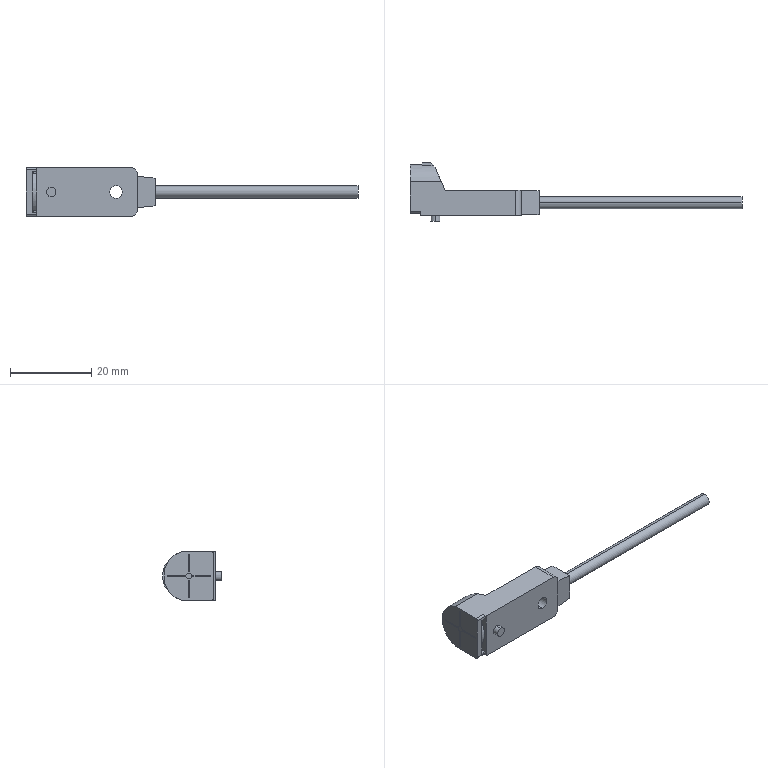Part | STEP file | gx-h12a | 1 solid | 70 faces | box 81.8 x 14.5 x 12 mm | volume 2908 mm3 | plane 49 | cylinder 20 | spline 1 | commonest cylinder face diameters 1.5 x4 3 x4 1 x2 2.3 x2 3.1 x2 6 x2